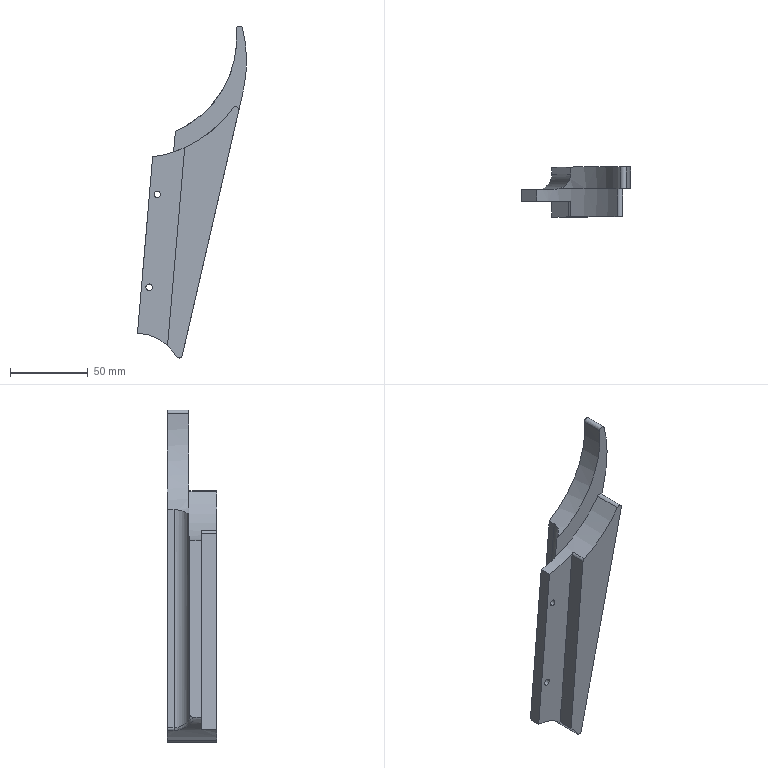Part | SolidWorks | features ICE 3, Fillet 2, DelFace 1, Extrusion 1, MirrorSolid 1 | 1 solid | 26 faces | box 70.208 x 32 x 213.495 mm | volume 127310 mm3 | cylinder 15 | plane 9 | spline 1 | torus 1 | commonest cylinder face diameters 4 x6 4.2 x4 20 x1 61 x1 130 x1 154 x1
STEP:
#1=CARTESIAN_POINT('',(13.896,-7.5,121.876));
#2=VERTEX_POINT('',#1);
#3=CARTESIAN_POINT('',(13.896,-7.5,117.676));
#4=VERTEX_POINT('',#3);
#5=CARTESIAN_POINT('',(13.896,-7.5,119.776));
#6=DIRECTION('',(0.,-1.,0.));
#7=DIRECTION('',(0.,0.,1.));
#8=AXIS2_PLACEMENT_3D('',#5,#6,#7);
#9=CIRCLE('',#8,2.1);
#10=EDGE_CURVE('',#2,#4,#9,.T.);
#11=ORIENTED_EDGE('',*,*,#10,.T.);
#12=CARTESIAN_POINT('',(13.896,0.,117.676));
#13=VERTEX_POINT('',#12);
#14=CARTESIAN_POINT('',(13.896,-148.287,117.676));
#15=DIRECTION('',(0.,1.,0.));
#16=VECTOR('',#15,1000.);
#17=LINE('',#14,#16);
#18=EDGE_CURVE('',#4,#13,#17,.T.);
#19=ORIENTED_EDGE('',*,*,#18,.T.);
#20=CARTESIAN_POINT('',(13.896,0.,121.876));
#21=VERTEX_POINT('',#20);
#22=CARTESIAN_POINT('',(13.896,0.,119.776));
#23=DIRECTION('',(0.,1.,0.));
#24=DIRECTION('',(0.,0.,1.));
#25=AXIS2_PLACEMENT_3D('',#22,#23,#24);
#26=CIRCLE('',#25,2.1);
#27=EDGE_CURVE('',#13,#21,#26,.T.);
#28=ORIENTED_EDGE('',*,*,#27,.T.);
#29=CARTESIAN_POINT('',(13.896,-148.287,121.876));
#30=DIRECTION('',(0.,1.,0.));
#31=VECTOR('',#30,1000.);
#32=LINE('',#29,#31);
#33=EDGE_CURVE('',#2,#21,#32,.T.);
#34=ORIENTED_EDGE('',*,*,#33,.F.);
#35=EDGE_LOOP('',(#11,#19,#28,#34));
#36=FACE_OUTER_BOUND('',#35,.T.);
#37=CARTESIAN_POINT('',(13.896,-148.287,119.776));
#38=DIRECTION('',(0.,1.,0.));
#39=DIRECTION('',(0.,0.,1.));
#40=AXIS2_PLACEMENT_3D('',#37,#38,#39);
#41=CYLINDRICAL_SURFACE('',#40,2.1);
#42=ADVANCED_FACE('',(#36),#41,.F.);
#43=CARTESIAN_POINT('',(8.714,-7.5,62.1));
#44=VERTEX_POINT('',#43);
#45=CARTESIAN_POINT('',(8.714,-7.5,57.9));
#46=VERTEX_POINT('',#45);
#47=CARTESIAN_POINT('',(8.714,-7.5,60.));
#48=DIRECTION('',(0.,-1.,0.));
#49=DIRECTION('',(0.,0.,1.));
#50=AXIS2_PLACEMENT_3D('',#47,#48,#49);
#51=CIRCLE('',#50,2.1);
#52=EDGE_CURVE('',#44,#46,#51,.T.);
#53=ORIENTED_EDGE('',*,*,#52,.T.);
#54=CARTESIAN_POINT('',(8.714,0.,57.9));
#55=VERTEX_POINT('',#54);
#56=CARTESIAN_POINT('',(8.714,-148.287,57.9));
#57=DIRECTION('',(0.,1.,0.));
#58=VECTOR('',#57,1000.);
#59=LINE('',#56,#58);
#60=EDGE_CURVE('',#46,#55,#59,.T.);
#61=ORIENTED_EDGE('',*,*,#60,.T.);
#62=CARTESIAN_POINT('',(8.714,0.,62.1));
#63=VERTEX_POINT('',#62);
#64=CARTESIAN_POINT('',(8.714,0.,60.));
#65=DIRECTION('',(0.,1.,0.));
#66=DIRECTION('',(0.,0.,1.));
#67=AXIS2_PLACEMENT_3D('',#64,#65,#66);
#68=CIRCLE('',#67,2.1);
#69=EDGE_CURVE('',#55,#63,#68,.T.);
#70=ORIENTED_EDGE('',*,*,#69,.T.);
#71=CARTESIAN_POINT('',(8.714,-148.287,62.1));
#72=DIRECTION('',(0.,1.,0.));
#73=VECTOR('',#72,1000.);
#74=LINE('',#71,#73);
#75=EDGE_CURVE('',#44,#63,#74,.T.);
#76=ORIENTED_EDGE('',*,*,#75,.F.);
#77=EDGE_LOOP('',(#53,#61,#70,#76));
#78=FACE_OUTER_BOUND('',#77,.T.);
#79=CARTESIAN_POINT('',(8.714,-148.287,60.));
#80=DIRECTION('',(0.,1.,0.));
#81=DIRECTION('',(0.,0.,1.));
#82=AXIS2_PLACEMENT_3D('',#79,#80,#81);
#83=CYLINDRICAL_SURFACE('',#82,2.1);
#84=ADVANCED_FACE('',(#78),#83,.F.);
#85=CARTESIAN_POINT('',(26.282,14.5,15.476));
#86=VERTEX_POINT('',#85);
#87=CARTESIAN_POINT('',(28.006,14.5,14.491));
#88=VERTEX_POINT('',#87);
#89=CARTESIAN_POINT('',(28.006,14.5,16.491));
#90=DIRECTION('',(0.,-1.,0.));
#91=DIRECTION('',(0.,0.,1.));
#92=AXIS2_PLACEMENT_3D('',#89,#90,#91);
#93=CIRCLE('',#92,2.);
#94=EDGE_CURVE('',#86,#88,#93,.T.);
#95=ORIENTED_EDGE('',*,*,#94,.T.);
#96=CARTESIAN_POINT('',(28.006,-17.5,14.491));
#97=VERTEX_POINT('',#96);
#98=CARTESIAN_POINT('',(28.006,17.5,14.491));
#99=DIRECTION('',(0.,-1.,0.));
#100=VECTOR('',#99,1000.);
#101=LINE('',#98,#100);
#102=EDGE_CURVE('',#88,#97,#101,.T.);
#103=ORIENTED_EDGE('',*,*,#102,.T.);
#104=CARTESIAN_POINT('',(26.282,-17.5,15.476));
#105=VERTEX_POINT('',#104);
#106=CARTESIAN_POINT('',(28.006,-17.5,16.491));
#107=DIRECTION('',(0.,-1.,0.));
#108=DIRECTION('',(0.,0.,1.));
#109=AXIS2_PLACEMENT_3D('',#106,#107,#108);
#110=CIRCLE('',#109,2.);
#111=EDGE_CURVE('',#105,#97,#110,.T.);
#112=ORIENTED_EDGE('',*,*,#111,.F.);
#113=CARTESIAN_POINT('',(26.282,17.5,15.476));
#114=DIRECTION('',(0.,-1.,0.));
#115=VECTOR('',#114,1000.);
#116=LINE('',#113,#115);
#117=EDGE_CURVE('',#86,#105,#116,.T.);
#118=ORIENTED_EDGE('',*,*,#117,.F.);
#119=EDGE_LOOP('',(#95,#103,#112,#118));
#120=FACE_OUTER_BOUND('',#119,.T.);
#121=CARTESIAN_POINT('',(28.006,17.5,16.491));
#122=DIRECTION('',(0.,-1.,0.));
#123=DIRECTION('',(0.,0.,-1.));
#124=AXIS2_PLACEMENT_3D('',#121,#122,#123);
#125=CYLINDRICAL_SURFACE('',#124,2.);
#126=ADVANCED_FACE('',(#120),#125,.T.);
#127=CARTESIAN_POINT('',(32.775,14.5,163.868));
#128=VERTEX_POINT('',#127);
#129=CARTESIAN_POINT('',(20.609,14.5,23.527));
#130=VERTEX_POINT('',#129);
#131=CARTESIAN_POINT('',(35.992,14.5,200.98));
#132=DIRECTION('',(-0.08636,0.,-0.9963));
#133=VECTOR('',#132,1000.);
#134=LINE('',#131,#133);
#135=EDGE_CURVE('',#128,#130,#134,.T.);
#136=ORIENTED_EDGE('',*,*,#135,.T.);
#137=CARTESIAN_POINT('',(20.609,10.,23.527));
#138=VERTEX_POINT('',#137);
#139=CARTESIAN_POINT('',(20.609,17.5,23.527));
#140=DIRECTION('',(0.,-1.,0.));
#141=VECTOR('',#140,1000.);
#142=LINE('',#139,#141);
#143=EDGE_CURVE('',#130,#138,#142,.T.);
#144=ORIENTED_EDGE('',*,*,#143,.T.);
#145=CARTESIAN_POINT('',(32.775,10.,163.868));
#146=VERTEX_POINT('',#145);
#147=CARTESIAN_POINT('',(20.525,10.,22.56));
#148=DIRECTION('',(0.08636,0.,0.9963));
#149=VECTOR('',#148,1000.);
#150=LINE('',#147,#149);
#151=EDGE_CURVE('',#138,#146,#150,.T.);
#152=ORIENTED_EDGE('',*,*,#151,.T.);
#153=CARTESIAN_POINT('',(32.775,0.5,163.868));
#154=DIRECTION('',(0.,1.,0.));
#155=VECTOR('',#154,1000.);
#156=LINE('',#153,#155);
#157=EDGE_CURVE('',#146,#128,#156,.T.);
#158=ORIENTED_EDGE('',*,*,#157,.T.);
#159=EDGE_LOOP('',(#136,#144,#152,#158));
#160=FACE_OUTER_BOUND('',#159,.T.);
#161=CARTESIAN_POINT('',(20.525,17.5,22.56));
#162=DIRECTION('',(0.9963,0.,-0.08636));
#163=DIRECTION('',(-0.08636,0.,-0.9963));
#164=AXIS2_PLACEMENT_3D('',#161,#162,#163);
#165=PLANE('',#164);
#166=ADVANCED_FACE('',(#160),#165,.F.);
#167=CARTESIAN_POINT('',(29.954,-17.5,16.041));
#168=VERTEX_POINT('',#167);
#169=CARTESIAN_POINT('',(29.954,14.5,16.041));
#170=VERTEX_POINT('',#169);
#171=CARTESIAN_POINT('',(29.954,17.5,16.041));
#172=DIRECTION('',(0.,1.,0.));
#173=VECTOR('',#172,1000.);
#174=LINE('',#171,#173);
#175=EDGE_CURVE('',#168,#170,#174,.T.);
#176=ORIENTED_EDGE('',*,*,#175,.T.);
#177=CARTESIAN_POINT('',(69.167,14.5,186.164));
#178=VERTEX_POINT('',#177);
#179=CARTESIAN_POINT('',(69.167,14.5,186.164));
#180=DIRECTION('',(0.2246,0.,0.9744));
#181=VECTOR('',#180,1000.);
#182=LINE('',#179,#181);
#183=EDGE_CURVE('',#170,#178,#182,.T.);
#184=ORIENTED_EDGE('',*,*,#183,.T.);
#185=CARTESIAN_POINT('',(69.167,0.5,186.164));
#186=VERTEX_POINT('',#185);
#187=CARTESIAN_POINT('',(69.167,0.5,186.164));
#188=DIRECTION('',(0.,1.,0.));
#189=VECTOR('',#188,1000.);
#190=LINE('',#187,#189);
#191=EDGE_CURVE('',#186,#178,#190,.T.);
#192=ORIENTED_EDGE('',*,*,#191,.F.);
#193=CARTESIAN_POINT('',(66.301,0.5,173.727));
#194=VERTEX_POINT('',#193);
#195=CARTESIAN_POINT('',(28.661,0.5,10.43));
#196=DIRECTION('',(-0.2246,0.,-0.9744));
#197=VECTOR('',#196,1000.);
#198=LINE('',#195,#197);
#199=EDGE_CURVE('',#186,#194,#198,.T.);
#200=ORIENTED_EDGE('',*,*,#199,.T.);
#201=CARTESIAN_POINT('',(66.301,-17.5,173.727));
#202=VERTEX_POINT('',#201);
#203=CARTESIAN_POINT('',(66.301,17.5,173.727));
#204=DIRECTION('',(0.,-1.,0.));
#205=VECTOR('',#204,1000.);
#206=LINE('',#203,#205);
#207=EDGE_CURVE('',#194,#202,#206,.T.);
#208=ORIENTED_EDGE('',*,*,#207,.T.);
#209=CARTESIAN_POINT('',(28.661,-17.5,10.43));
#210=DIRECTION('',(-0.2246,0.,-0.9744));
#211=VECTOR('',#210,1000.);
#212=LINE('',#209,#211);
#213=EDGE_CURVE('',#202,#168,#212,.T.);
#214=ORIENTED_EDGE('',*,*,#213,.T.);
#215=EDGE_LOOP('',(#176,#184,#192,#200,#208,#214));
#216=FACE_OUTER_BOUND('',#215,.T.);
#217=CARTESIAN_POINT('',(28.661,17.5,10.43));
#218=DIRECTION('',(-0.9744,0.,0.2246));
#219=DIRECTION('',(0.2246,0.,0.9744));
#220=AXIS2_PLACEMENT_3D('',#217,#218,#219);
#221=PLANE('',#220);
#222=ADVANCED_FACE('',(#216),#221,.F.);
#223=CARTESIAN_POINT('',(21.211,14.5,21.917));
#224=VERTEX_POINT('',#223);
#225=CARTESIAN_POINT('',(0.,14.5,0.));
#226=DIRECTION('',(0.,1.,0.));
#227=DIRECTION('',(0.,0.,1.));
#228=AXIS2_PLACEMENT_3D('',#225,#226,#227);
#229=CIRCLE('',#228,30.5);
#230=EDGE_CURVE('',#224,#86,#229,.T.);
#231=ORIENTED_EDGE('',*,*,#230,.T.);
#232=ORIENTED_EDGE('',*,*,#117,.T.);
#233=CARTESIAN_POINT('',(20.525,-17.5,22.56));
#234=VERTEX_POINT('',#233);
#235=CARTESIAN_POINT('',(0.,-17.5,0.));
#236=DIRECTION('',(0.,-1.,0.));
#237=DIRECTION('',(0.,0.,1.));
#238=AXIS2_PLACEMENT_3D('',#235,#236,#237);
#239=CIRCLE('',#238,30.5);
#240=EDGE_CURVE('',#105,#234,#239,.T.);
#241=ORIENTED_EDGE('',*,*,#240,.T.);
#242=CARTESIAN_POINT('',(20.525,-7.5,22.56));
#243=VERTEX_POINT('',#242);
#244=CARTESIAN_POINT('',(20.525,17.5,22.56));
#245=DIRECTION('',(0.,-1.,0.));
#246=VECTOR('',#245,1000.);
#247=LINE('',#244,#246);
#248=EDGE_CURVE('',#243,#234,#247,.T.);
#249=ORIENTED_EDGE('',*,*,#248,.F.);
#250=CARTESIAN_POINT('',(1.137,-7.5,30.479));
#251=VERTEX_POINT('',#250);
#252=CARTESIAN_POINT('',(0.,-7.5,0.));
#253=DIRECTION('',(0.,1.,0.));
#254=DIRECTION('',(0.,0.,1.));
#255=AXIS2_PLACEMENT_3D('',#252,#253,#254);
#256=CIRCLE('',#255,30.5);
#257=EDGE_CURVE('',#251,#243,#256,.T.);
#258=ORIENTED_EDGE('',*,*,#257,.F.);
#259=CARTESIAN_POINT('',(1.137,-2.,30.479));
#260=VERTEX_POINT('',#259);
#261=CARTESIAN_POINT('',(1.137,-148.287,30.479));
#262=DIRECTION('',(0.,1.,0.));
#263=VECTOR('',#262,1000.);
#264=LINE('',#261,#263);
#265=EDGE_CURVE('',#251,#260,#264,.T.);
#266=ORIENTED_EDGE('',*,*,#265,.T.);
#267=CARTESIAN_POINT('',(10.49,-2.,28.639));
#268=VERTEX_POINT('',#267);
#269=CARTESIAN_POINT('',(0.,-2.,0.));
#270=DIRECTION('',(0.,1.,0.));
#271=DIRECTION('',(0.,0.,1.));
#272=AXIS2_PLACEMENT_3D('',#269,#270,#271);
#273=CIRCLE('',#272,30.5);
#274=EDGE_CURVE('',#260,#268,#273,.T.);
#275=ORIENTED_EDGE('',*,*,#274,.T.);
#276=CARTESIAN_POINT('',(21.211,10.,21.917));
#277=VERTEX_POINT('',#276);
#278=CARTESIAN_POINT('',(10.49,-2.,28.639));
#279=CARTESIAN_POINT('',(11.252,-2.,28.36));
#280=CARTESIAN_POINT('',(11.986,-1.914,28.057));
#281=CARTESIAN_POINT('',(13.052,-1.671,27.569));
#282=CARTESIAN_POINT('',(13.401,-1.571,27.401));
#283=CARTESIAN_POINT('',(14.087,-1.333,27.054));
#284=CARTESIAN_POINT('',(14.425,-1.194,26.876));
#285=CARTESIAN_POINT('',(15.401,-0.7323,26.337));
#286=CARTESIAN_POINT('',(16.007,-0.3609,25.971));
#287=CARTESIAN_POINT('',(16.858,0.2868,25.42));
#288=CARTESIAN_POINT('',(17.133,0.5188,25.235));
#289=CARTESIAN_POINT('',(17.659,1.01,24.87));
#290=CARTESIAN_POINT('',(17.909,1.268,24.69));
#291=CARTESIAN_POINT('',(18.621,2.077,24.163));
#292=CARTESIAN_POINT('',(19.046,2.663,23.827));
#293=CARTESIAN_POINT('',(19.611,3.618,23.36));
#294=CARTESIAN_POINT('',(19.789,3.951,23.21));
#295=CARTESIAN_POINT('',(20.112,4.635,22.93));
#296=CARTESIAN_POINT('',(20.259,4.985,22.8));
#297=CARTESIAN_POINT('',(20.523,5.703,22.563));
#298=CARTESIAN_POINT('',(20.641,6.071,22.455));
#299=CARTESIAN_POINT('',(20.844,6.825,22.266));
#300=CARTESIAN_POINT('',(20.931,7.214,22.184));
#301=CARTESIAN_POINT('',(21.14,8.391,21.986));
#302=CARTESIAN_POINT('',(21.211,9.188,21.917));
#303=CARTESIAN_POINT('',(21.211,10.,21.917));
#304=B_SPLINE_CURVE_WITH_KNOTS('',3,(#278,#279,#280,#281,#282,#283,#284,#285,#286,#287,#288,#289,#290,#291,#292,#293,#294,#295,#296,#297,#298,#299,#300,#301,#302,#303),.UNSPECIFIED.,.F.,.F.,(4,2,2,2,2,2,2,2,2,2,2,2,4),(0.,0.002393,0.003589,0.004785,0.007178,0.008374,0.009571,0.01196,0.01316,0.01436,0.01555,0.01675,0.01914),.UNSPECIFIED.);
#305=EDGE_CURVE('',#268,#277,#304,.T.);
#306=ORIENTED_EDGE('',*,*,#305,.T.);
#307=CARTESIAN_POINT('',(21.211,17.5,21.917));
#308=DIRECTION('',(0.,1.,0.));
#309=VECTOR('',#308,1000.);
#310=LINE('',#307,#309);
#311=EDGE_CURVE('',#277,#224,#310,.T.);
#312=ORIENTED_EDGE('',*,*,#311,.T.);
#313=EDGE_LOOP('',(#231,#232,#241,#249,#258,#266,#275,#306,#312));
#314=FACE_OUTER_BOUND('',#313,.T.);
#315=CARTESIAN_POINT('',(0.,17.5,0.));
#316=DIRECTION('',(0.,-1.,0.));
#317=DIRECTION('',(0.,0.,-1.));
#318=AXIS2_PLACEMENT_3D('',#315,#316,#317);
#319=CYLINDRICAL_SURFACE('',#318,30.5);
#320=ADVANCED_FACE('',(#314),#319,.F.);
#321=ORIENTED_EDGE('',*,*,#143,.F.);
#322=CARTESIAN_POINT('',(22.601,14.5,23.354));
#323=DIRECTION('',(0.,-1.,0.));
#324=DIRECTION('',(0.,0.,1.));
#325=AXIS2_PLACEMENT_3D('',#322,#323,#324);
#326=CIRCLE('',#325,2.);
#327=EDGE_CURVE('',#130,#224,#326,.T.);
#328=ORIENTED_EDGE('',*,*,#327,.T.);
#329=ORIENTED_EDGE('',*,*,#311,.F.);
#330=CARTESIAN_POINT('',(22.601,10.,23.354));
#331=DIRECTION('',(0.,-1.,0.));
#332=DIRECTION('',(0.,0.,-1.));
#333=AXIS2_PLACEMENT_3D('',#330,#331,#332);
#334=CIRCLE('',#333,2.);
#335=EDGE_CURVE('',#138,#277,#334,.T.);
#336=ORIENTED_EDGE('',*,*,#335,.F.);
#337=EDGE_LOOP('',(#321,#328,#329,#336));
#338=FACE_OUTER_BOUND('',#337,.T.);
#339=CARTESIAN_POINT('',(22.601,17.5,23.354));
#340=DIRECTION('',(0.,-1.,0.));
#341=DIRECTION('',(0.,0.,-1.));
#342=AXIS2_PLACEMENT_3D('',#339,#340,#341);
#343=CYLINDRICAL_SURFACE('',#342,2.);
#344=ADVANCED_FACE('',(#338),#343,.T.);
#345=ORIENTED_EDGE('',*,*,#102,.F.);
#346=CARTESIAN_POINT('',(28.006,14.5,16.491));
#347=DIRECTION('',(0.,-1.,0.));
#348=DIRECTION('',(0.,0.,1.));
#349=AXIS2_PLACEMENT_3D('',#346,#347,#348);
#350=CIRCLE('',#349,2.);
#351=EDGE_CURVE('',#88,#170,#350,.T.);
#352=ORIENTED_EDGE('',*,*,#351,.T.);
#353=ORIENTED_EDGE('',*,*,#175,.F.);
#354=CARTESIAN_POINT('',(28.006,-17.5,16.491));
#355=DIRECTION('',(0.,-1.,0.));
#356=DIRECTION('',(0.,0.,1.));
#357=AXIS2_PLACEMENT_3D('',#354,#355,#356);
#358=CIRCLE('',#357,2.);
#359=EDGE_CURVE('',#97,#168,#358,.T.);
#360=ORIENTED_EDGE('',*,*,#359,.F.);
#361=EDGE_LOOP('',(#345,#352,#353,#360));
#362=FACE_OUTER_BOUND('',#361,.T.);
#363=CARTESIAN_POINT('',(28.006,17.5,16.491));
#364=DIRECTION('',(0.,-1.,0.));
#365=DIRECTION('',(0.,0.,-1.));
#366=AXIS2_PLACEMENT_3D('',#363,#364,#365);
#367=CYLINDRICAL_SURFACE('',#366,2.);
#368=ADVANCED_FACE('',(#362),#367,.T.);
#369=CARTESIAN_POINT('',(32.597,-17.5,150.24));
#370=VERTEX_POINT('',#369);
#371=CARTESIAN_POINT('',(62.723,-17.5,175.336));
#372=VERTEX_POINT('',#371);
#373=CARTESIAN_POINT('',(0.,-17.5,220.));
#374=DIRECTION('',(0.,-1.,0.));
#375=DIRECTION('',(0.,0.,1.));
#376=AXIS2_PLACEMENT_3D('',#373,#374,#375);
#377=CIRCLE('',#376,77.);
#378=EDGE_CURVE('',#370,#372,#377,.T.);
#379=ORIENTED_EDGE('',*,*,#378,.T.);
#380=CARTESIAN_POINT('',(62.723,0.5,175.336));
#381=VERTEX_POINT('',#380);
#382=CARTESIAN_POINT('',(62.723,17.5,175.336));
#383=DIRECTION('',(0.,1.,0.));
#384=VECTOR('',#383,1000.);
#385=LINE('',#382,#384);
#386=EDGE_CURVE('',#372,#381,#385,.T.);
#387=ORIENTED_EDGE('',*,*,#386,.T.);
#388=CARTESIAN_POINT('',(24.407,0.5,146.97));
#389=VERTEX_POINT('',#388);
#390=CARTESIAN_POINT('',(0.,0.5,220.));
#391=DIRECTION('',(0.,1.,0.));
#392=DIRECTION('',(0.,0.,1.));
#393=AXIS2_PLACEMENT_3D('',#390,#391,#392);
#394=CIRCLE('',#393,77.);
#395=EDGE_CURVE('',#381,#389,#394,.T.);
#396=ORIENTED_EDGE('',*,*,#395,.T.);
#397=CARTESIAN_POINT('',(21.186,0.,145.972));
#398=VERTEX_POINT('',#397);
#399=CARTESIAN_POINT('',(24.407,0.5,146.97));
#400=CARTESIAN_POINT('',(23.364,0.1684,146.622));
#401=CARTESIAN_POINT('',(22.291,0.,146.288));
#402=CARTESIAN_POINT('',(21.186,0.,145.972));
#403=B_SPLINE_CURVE_WITH_KNOTS('',3,(#399,#400,#401,#402),.UNSPECIFIED.,.F.,.F.,(4,4),(0.01301,0.01641),.UNSPECIFIED.);
#404=EDGE_CURVE('',#389,#398,#403,.T.);
#405=ORIENTED_EDGE('',*,*,#404,.T.);
#406=CARTESIAN_POINT('',(10.959,0.,143.784));
#407=VERTEX_POINT('',#406);
#408=CARTESIAN_POINT('',(0.,0.,220.));
#409=DIRECTION('',(0.,-1.,0.));
#410=DIRECTION('',(0.,0.,1.));
#411=AXIS2_PLACEMENT_3D('',#408,#409,#410);
#412=CIRCLE('',#411,77.);
#413=EDGE_CURVE('',#407,#398,#412,.T.);
#414=ORIENTED_EDGE('',*,*,#413,.F.);
#415=CARTESIAN_POINT('',(10.959,-7.5,143.784));
#416=VERTEX_POINT('',#415);
#417=CARTESIAN_POINT('',(10.959,-148.287,143.784));
#418=DIRECTION('',(0.,1.,0.));
#419=VECTOR('',#418,1000.);
#420=LINE('',#417,#419);
#421=EDGE_CURVE('',#416,#407,#420,.T.);
#422=ORIENTED_EDGE('',*,*,#421,.F.);
#423=CARTESIAN_POINT('',(32.597,-7.5,150.24));
#424=VERTEX_POINT('',#423);
#425=CARTESIAN_POINT('',(0.,-7.5,220.));
#426=DIRECTION('',(0.,1.,0.));
#427=DIRECTION('',(0.,0.,1.));
#428=AXIS2_PLACEMENT_3D('',#425,#426,#427);
#429=CIRCLE('',#428,77.);
#430=EDGE_CURVE('',#424,#416,#429,.T.);
#431=ORIENTED_EDGE('',*,*,#430,.F.);
#432=CARTESIAN_POINT('',(32.597,17.5,150.24));
#433=DIRECTION('',(0.,-1.,0.));
#434=VECTOR('',#433,1000.);
#435=LINE('',#432,#434);
#436=EDGE_CURVE('',#424,#370,#435,.T.);
#437=ORIENTED_EDGE('',*,*,#436,.T.);
#438=EDGE_LOOP('',(#379,#387,#396,#405,#414,#422,#431,#437));
#439=FACE_OUTER_BOUND('',#438,.T.);
#440=CARTESIAN_POINT('',(0.,17.5,220.));
#441=DIRECTION('',(0.,-1.,0.));
#442=DIRECTION('',(0.,0.,-1.));
#443=AXIS2_PLACEMENT_3D('',#440,#441,#442);
#444=CYLINDRICAL_SURFACE('',#443,77.);
#445=ADVANCED_FACE('',(#439),#444,.F.);
#446=CARTESIAN_POINT('',(31.451,-17.5,148.601));
#447=VERTEX_POINT('',#446);
#448=CARTESIAN_POINT('',(20.525,-17.5,22.56));
#449=DIRECTION('',(0.08636,0.,0.9963));
#450=VECTOR('',#449,1000.);
#451=LINE('',#448,#450);
#452=EDGE_CURVE('',#234,#447,#451,.T.);
#453=ORIENTED_EDGE('',*,*,#452,.T.);
#454=CARTESIAN_POINT('',(31.451,-7.5,148.601));
#455=VERTEX_POINT('',#454);
#456=CARTESIAN_POINT('',(31.451,17.5,148.601));
#457=DIRECTION('',(0.,1.,0.));
#458=VECTOR('',#457,1000.);
#459=LINE('',#456,#458);
#460=EDGE_CURVE('',#447,#455,#459,.T.);
#461=ORIENTED_EDGE('',*,*,#460,.T.);
#462=CARTESIAN_POINT('',(20.525,-7.5,22.56));
#463=DIRECTION('',(0.08636,0.,0.9963));
#464=VECTOR('',#463,1000.);
#465=LINE('',#462,#464);
#466=EDGE_CURVE('',#243,#455,#465,.T.);
#467=ORIENTED_EDGE('',*,*,#466,.F.);
#468=ORIENTED_EDGE('',*,*,#248,.T.);
#469=EDGE_LOOP('',(#453,#461,#467,#468));
#470=FACE_OUTER_BOUND('',#469,.T.);
#471=CARTESIAN_POINT('',(20.525,17.5,22.56));
#472=DIRECTION('',(0.9963,0.,-0.08636));
#473=DIRECTION('',(-0.08636,0.,-0.9963));
#474=AXIS2_PLACEMENT_3D('',#471,#472,#473);
#475=PLANE('',#474);
#476=ADVANCED_FACE('',(#470),#475,.F.);
#477=ORIENTED_EDGE('',*,*,#213,.F.);
#478=CARTESIAN_POINT('',(64.352,-17.5,174.176));
#479=DIRECTION('',(0.,-1.,0.));
#480=DIRECTION('',(0.,0.,1.));
#481=AXIS2_PLACEMENT_3D('',#478,#479,#480);
#482=CIRCLE('',#481,2.);
#483=EDGE_CURVE('',#202,#372,#482,.T.);
#484=ORIENTED_EDGE('',*,*,#483,.T.);
#485=ORIENTED_EDGE('',*,*,#378,.F.);
#486=CARTESIAN_POINT('',(33.444,-17.5,148.428));
#487=DIRECTION('',(0.,-1.,0.));
#488=DIRECTION('',(0.,0.,1.));
#489=AXIS2_PLACEMENT_3D('',#486,#487,#488);
#490=CIRCLE('',#489,2.);
#491=EDGE_CURVE('',#370,#447,#490,.T.);
#492=ORIENTED_EDGE('',*,*,#491,.T.);
#493=ORIENTED_EDGE('',*,*,#452,.F.);
#494=ORIENTED_EDGE('',*,*,#240,.F.);
#495=ORIENTED_EDGE('',*,*,#111,.T.);
#496=ORIENTED_EDGE('',*,*,#359,.T.);
#497=EDGE_LOOP('',(#477,#484,#485,#492,#493,#494,#495,#496));
#498=FACE_OUTER_BOUND('',#497,.T.);
#499=CARTESIAN_POINT('',(0.,-17.5,220.));
#500=DIRECTION('',(0.,1.,0.));
#501=DIRECTION('',(0.,0.,1.));
#502=AXIS2_PLACEMENT_3D('',#499,#500,#501);
#503=PLANE('',#502);
#504=ADVANCED_FACE('',(#498),#503,.F.);
#505=CARTESIAN_POINT('',(1.309,0.,32.474));
#506=VERTEX_POINT('',#505);
#507=CARTESIAN_POINT('',(1.137,0.,30.479));
#508=DIRECTION('',(0.08636,0.,0.9963));
#509=VECTOR('',#508,1000.);
#510=LINE('',#507,#509);
#511=EDGE_CURVE('',#506,#407,#510,.T.);
#512=ORIENTED_EDGE('',*,*,#511,.F.);
#513=CARTESIAN_POINT('',(1.309,0.,32.474));
#514=CARTESIAN_POINT('',(1.298,0.,32.342));
#515=CARTESIAN_POINT('',(1.287,-0.01294,32.213));
#516=CARTESIAN_POINT('',(1.265,-0.06363,31.958));
#517=CARTESIAN_POINT('',(1.254,-0.102,31.831));
#518=CARTESIAN_POINT('',(1.233,-0.2022,31.59));
#519=CARTESIAN_POINT('',(1.223,-0.2635,31.475));
#520=CARTESIAN_POINT('',(1.204,-0.4084,31.259));
#521=CARTESIAN_POINT('',(1.195,-0.4927,31.156));
#522=CARTESIAN_POINT('',(1.171,-0.7692,30.88));
#523=CARTESIAN_POINT('',(1.158,-0.9921,30.731));
#524=CARTESIAN_POINT('',(1.141,-1.473,30.532));
#525=CARTESIAN_POINT('',(1.137,-1.736,30.479));
#526=CARTESIAN_POINT('',(1.137,-2.,30.479));
#527=B_SPLINE_CURVE_WITH_KNOTS('',3,(#513,#514,#515,#516,#517,#518,#519,#520,#521,#522,#523,#524,#525,#526),.UNSPECIFIED.,.F.,.F.,(4,2,2,2,2,2,4),(0.,0.0003908,0.0007815,0.001172,0.001563,0.002345,0.003126),.UNSPECIFIED.);
#528=EDGE_CURVE('',#506,#260,#527,.T.);
#529=ORIENTED_EDGE('',*,*,#528,.T.);
#530=ORIENTED_EDGE('',*,*,#265,.F.);
#531=CARTESIAN_POINT('',(1.137,-7.5,30.479));
#532=DIRECTION('',(-0.08636,0.,-0.9963));
#533=VECTOR('',#532,1000.);
#534=LINE('',#531,#533);
#535=EDGE_CURVE('',#416,#251,#534,.T.);
#536=ORIENTED_EDGE('',*,*,#535,.F.);
#537=ORIENTED_EDGE('',*,*,#421,.T.);
#538=EDGE_LOOP('',(#512,#529,#530,#536,#537));
#539=FACE_OUTER_BOUND('',#538,.T.);
#540=CARTESIAN_POINT('',(1.137,-148.287,30.479));
#541=DIRECTION('',(-0.9963,0.,0.08636));
#542=DIRECTION('',(0.08636,0.,0.9963));
#543=AXIS2_PLACEMENT_3D('',#540,#541,#542);
#544=PLANE('',#543);
#545=ADVANCED_FACE('',(#539),#544,.T.);
#546=ORIENTED_EDGE('',*,*,#60,.F.);
#547=CARTESIAN_POINT('',(8.714,-7.5,60.));
#548=DIRECTION('',(0.,-1.,0.));
#549=DIRECTION('',(0.,0.,1.));
#550=AXIS2_PLACEMENT_3D('',#547,#548,#549);
#551=CIRCLE('',#550,2.1);
#552=EDGE_CURVE('',#46,#44,#551,.T.);
#553=ORIENTED_EDGE('',*,*,#552,.T.);
#554=ORIENTED_EDGE('',*,*,#75,.T.);
#555=CARTESIAN_POINT('',(8.714,0.,60.));
#556=DIRECTION('',(0.,1.,0.));
#557=DIRECTION('',(0.,0.,1.));
#558=AXIS2_PLACEMENT_3D('',#555,#556,#557);
#559=CIRCLE('',#558,2.1);
#560=EDGE_CURVE('',#63,#55,#559,.T.);
#561=ORIENTED_EDGE('',*,*,#560,.T.);
#562=EDGE_LOOP('',(#546,#553,#554,#561));
#563=FACE_OUTER_BOUND('',#562,.T.);
#564=CARTESIAN_POINT('',(8.714,-148.287,60.));
#565=DIRECTION('',(0.,1.,0.));
#566=DIRECTION('',(0.,0.,1.));
#567=AXIS2_PLACEMENT_3D('',#564,#565,#566);
#568=CYLINDRICAL_SURFACE('',#567,2.1);
#569=ADVANCED_FACE('',(#563),#568,.F.);
#570=CARTESIAN_POINT('',(13.896,0.,119.776));
#571=DIRECTION('',(0.,1.,0.));
#572=DIRECTION('',(0.,0.,1.));
#573=AXIS2_PLACEMENT_3D('',#570,#571,#572);
#574=CIRCLE('',#573,2.1);
#575=EDGE_CURVE('',#21,#13,#574,.T.);
#576=ORIENTED_EDGE('',*,*,#575,.F.);
#577=ORIENTED_EDGE('',*,*,#27,.F.);
#578=EDGE_LOOP('',(#576,#577));
#579=FACE_BOUND('',#578,.T.);
#580=ORIENTED_EDGE('',*,*,#560,.F.);
#581=ORIENTED_EDGE('',*,*,#69,.F.);
#582=EDGE_LOOP('',(#580,#581));
#583=FACE_BOUND('',#582,.T.);
#584=CARTESIAN_POINT('',(11.177,0.,30.517));
#585=VERTEX_POINT('',#584);
#586=CARTESIAN_POINT('',(8.468,0.,-0.7341));
#587=DIRECTION('',(-0.08636,0.,-0.9963));
#588=VECTOR('',#587,1000.);
#589=LINE('',#586,#588);
#590=EDGE_CURVE('',#398,#585,#589,.T.);
#591=ORIENTED_EDGE('',*,*,#590,.T.);
#592=CARTESIAN_POINT('',(0.,0.,0.));
#593=DIRECTION('',(0.,-1.,0.));
#594=DIRECTION('',(0.,0.,1.));
#595=AXIS2_PLACEMENT_3D('',#592,#593,#594);
#596=CIRCLE('',#595,32.5);
#597=EDGE_CURVE('',#585,#506,#596,.T.);
#598=ORIENTED_EDGE('',*,*,#597,.T.);
#599=ORIENTED_EDGE('',*,*,#511,.T.);
#600=ORIENTED_EDGE('',*,*,#413,.T.);
#601=EDGE_LOOP('',(#591,#598,#599,#600));
#602=FACE_OUTER_BOUND('',#601,.T.);
#603=CARTESIAN_POINT('',(0.,0.,0.));
#604=DIRECTION('',(0.,1.,0.));
#605=DIRECTION('',(0.,0.,1.));
#606=AXIS2_PLACEMENT_3D('',#603,#604,#605);
#607=PLANE('',#606);
#608=ADVANCED_FACE('',(#579,#583,#602),#607,.T.);
#609=ORIENTED_EDGE('',*,*,#18,.F.);
#610=CARTESIAN_POINT('',(13.896,-7.5,119.776));
#611=DIRECTION('',(0.,-1.,0.));
#612=DIRECTION('',(0.,0.,1.));
#613=AXIS2_PLACEMENT_3D('',#610,#611,#612);
#614=CIRCLE('',#613,2.1);
#615=EDGE_CURVE('',#4,#2,#614,.T.);
#616=ORIENTED_EDGE('',*,*,#615,.T.);
#617=ORIENTED_EDGE('',*,*,#33,.T.);
#618=ORIENTED_EDGE('',*,*,#575,.T.);
#619=EDGE_LOOP('',(#609,#616,#617,#618));
#620=FACE_OUTER_BOUND('',#619,.T.);
#621=CARTESIAN_POINT('',(13.896,-148.287,119.776));
#622=DIRECTION('',(0.,1.,0.));
#623=DIRECTION('',(0.,0.,1.));
#624=AXIS2_PLACEMENT_3D('',#621,#622,#623);
#625=CYLINDRICAL_SURFACE('',#624,2.1);
#626=ADVANCED_FACE('',(#620),#625,.F.);
#627=ORIENTED_EDGE('',*,*,#257,.T.);
#628=ORIENTED_EDGE('',*,*,#466,.T.);
#629=CARTESIAN_POINT('',(33.444,-7.5,148.428));
#630=DIRECTION('',(0.,1.,0.));
#631=DIRECTION('',(0.,0.,1.));
#632=AXIS2_PLACEMENT_3D('',#629,#630,#631);
#633=CIRCLE('',#632,2.);
#634=EDGE_CURVE('',#455,#424,#633,.T.);
#635=ORIENTED_EDGE('',*,*,#634,.T.);
#636=ORIENTED_EDGE('',*,*,#430,.T.);
#637=ORIENTED_EDGE('',*,*,#535,.T.);
#638=EDGE_LOOP('',(#627,#628,#635,#636,#637));
#639=FACE_OUTER_BOUND('',#638,.T.);
#640=ORIENTED_EDGE('',*,*,#10,.F.);
#641=ORIENTED_EDGE('',*,*,#615,.F.);
#642=EDGE_LOOP('',(#640,#641));
#643=FACE_BOUND('',#642,.T.);
#644=ORIENTED_EDGE('',*,*,#52,.F.);
#645=ORIENTED_EDGE('',*,*,#552,.F.);
#646=EDGE_LOOP('',(#644,#645));
#647=FACE_BOUND('',#646,.T.);
#648=CARTESIAN_POINT('',(0.,-7.5,220.));
#649=DIRECTION('',(0.,1.,0.));
#650=DIRECTION('',(0.,0.,1.));
#651=AXIS2_PLACEMENT_3D('',#648,#649,#650);
#652=PLANE('',#651);
#653=ADVANCED_FACE('',(#639,#643,#647),#652,.F.);
#654=ORIENTED_EDGE('',*,*,#151,.F.);
#655=CARTESIAN_POINT('',(20.609,10.,23.527));
#656=CARTESIAN_POINT('',(20.609,9.283,23.527));
#657=CARTESIAN_POINT('',(20.539,8.582,23.609));
#658=CARTESIAN_POINT('',(20.338,7.556,23.837));
#659=CARTESIAN_POINT('',(20.254,7.22,23.931));
#660=CARTESIAN_POINT('',(20.061,6.574,24.145));
#661=CARTESIAN_POINT('',(19.951,6.261,24.265));
#662=CARTESIAN_POINT('',(19.704,5.654,24.528));
#663=CARTESIAN_POINT('',(19.568,5.36,24.671));
#664=CARTESIAN_POINT('',(19.27,4.788,24.977));
#665=CARTESIAN_POINT('',(19.109,4.514,25.138));
#666=CARTESIAN_POINT('',(18.599,3.729,25.635));
#667=CARTESIAN_POINT('',(18.219,3.252,25.988));
#668=CARTESIAN_POINT('',(17.38,2.381,26.718));
#669=CARTESIAN_POINT('',(16.916,1.985,27.097));
#670=CARTESIAN_POINT('',(15.931,1.298,27.843));
#671=CARTESIAN_POINT('',(15.407,1.004,28.212));
#672=CARTESIAN_POINT('',(14.566,0.6377,28.753));
#673=CARTESIAN_POINT('',(14.275,0.5283,28.932));
#674=CARTESIAN_POINT('',(13.686,0.3402,29.279));
#675=CARTESIAN_POINT('',(13.386,0.261,29.447));
#676=CARTESIAN_POINT('',(12.469,0.06853,29.935));
#677=CARTESIAN_POINT('',(11.836,0.,30.238));
#678=CARTESIAN_POINT('',(11.177,0.,30.517));
#679=B_SPLINE_CURVE_WITH_KNOTS('',3,(#655,#656,#657,#658,#659,#660,#661,#662,#663,#664,#665,#666,#667,#668,#669,#670,#671,#672,#673,#674,#675,#676,#677,#678),.UNSPECIFIED.,.F.,.F.,(4,2,2,2,2,2,2,2,2,2,2,4),(0.,0.002125,0.003187,0.004249,0.005311,0.006374,0.008498,0.01062,0.01275,0.01381,0.01487,0.017),.UNSPECIFIED.);
#680=EDGE_CURVE('',#138,#585,#679,.T.);
#681=ORIENTED_EDGE('',*,*,#680,.T.);
#682=ORIENTED_EDGE('',*,*,#590,.F.);
#683=ORIENTED_EDGE('',*,*,#404,.F.);
#684=CARTESIAN_POINT('',(25.556,0.5,160.235));
#685=VERTEX_POINT('',#684);
#686=CARTESIAN_POINT('',(11.579,0.5,-1.004));
#687=DIRECTION('',(0.08636,0.,0.9963));
#688=VECTOR('',#687,1000.);
#689=LINE('',#686,#688);
#690=EDGE_CURVE('',#389,#685,#689,.T.);
#691=ORIENTED_EDGE('',*,*,#690,.T.);
#692=CARTESIAN_POINT('',(25.556,0.5,160.235));
#693=CARTESIAN_POINT('',(26.546,0.8121,160.658));
#694=CARTESIAN_POINT('',(27.469,1.256,161.082));
#695=CARTESIAN_POINT('',(28.542,1.981,161.602));
#696=CARTESIAN_POINT('',(28.753,2.135,161.705));
#697=CARTESIAN_POINT('',(29.161,2.456,161.908));
#698=CARTESIAN_POINT('',(29.359,2.625,162.008));
#699=CARTESIAN_POINT('',(29.933,3.152,162.301));
#700=CARTESIAN_POINT('',(30.291,3.533,162.488));
#701=CARTESIAN_POINT('',(30.788,4.154,162.754));
#702=CARTESIAN_POINT('',(30.947,4.369,162.84));
#703=CARTESIAN_POINT('',(31.246,4.811,163.003));
#704=CARTESIAN_POINT('',(31.387,5.037,163.08));
#705=CARTESIAN_POINT('',(31.651,5.504,163.227));
#706=CARTESIAN_POINT('',(31.774,5.743,163.295));
#707=CARTESIAN_POINT('',(32.001,6.235,163.423));
#708=CARTESIAN_POINT('',(32.106,6.489,163.483));
#709=CARTESIAN_POINT('',(32.388,7.264,163.643));
#710=CARTESIAN_POINT('',(32.531,7.794,163.726));
#711=CARTESIAN_POINT('',(32.676,8.609,163.81));
#712=CARTESIAN_POINT('',(32.713,8.885,163.832));
#713=CARTESIAN_POINT('',(32.762,9.442,163.861));
#714=CARTESIAN_POINT('',(32.775,9.723,163.868));
#715=CARTESIAN_POINT('',(32.775,10.,163.868));
#716=B_SPLINE_CURVE_WITH_KNOTS('',3,(#692,#693,#694,#695,#696,#697,#698,#699,#700,#701,#702,#703,#704,#705,#706,#707,#708,#709,#710,#711,#712,#713,#714,#715),.UNSPECIFIED.,.F.,.F.,(4,2,2,2,2,2,2,2,2,2,2,4),(0.007444,0.01078,0.01161,0.01244,0.01411,0.01494,0.01577,0.01661,0.01744,0.01911,0.01994,0.02077),.UNSPECIFIED.);
#717=EDGE_CURVE('',#685,#146,#716,.T.);
#718=ORIENTED_EDGE('',*,*,#717,.T.);
#719=EDGE_LOOP('',(#654,#681,#682,#683,#691,#718));
#720=FACE_OUTER_BOUND('',#719,.T.);
#721=CARTESIAN_POINT('',(8.468,10.,-0.7341));
#722=DIRECTION('',(-0.08636,0.,-0.9963));
#723=DIRECTION('',(-0.9963,0.,0.08636));
#724=AXIS2_PLACEMENT_3D('',#721,#722,#723);
#725=CYLINDRICAL_SURFACE('',#724,10.);
#726=ADVANCED_FACE('',(#720),#725,.F.);
#727=CARTESIAN_POINT('',(68.669,14.5,226.483));
#728=VERTEX_POINT('',#727);
#729=CARTESIAN_POINT('',(-13.856,14.5,205.301));
#730=DIRECTION('',(0.,1.,0.));
#731=DIRECTION('',(0.,0.,1.));
#732=AXIS2_PLACEMENT_3D('',#729,#730,#731);
#733=CIRCLE('',#732,85.2);
#734=EDGE_CURVE('',#728,#178,#733,.T.);
#735=ORIENTED_EDGE('',*,*,#734,.F.);
#736=CARTESIAN_POINT('',(68.669,0.5,226.483));
#737=VERTEX_POINT('',#736);
#738=CARTESIAN_POINT('',(68.669,0.5,226.483));
#739=DIRECTION('',(0.,-1.,0.));
#740=VECTOR('',#739,1000.);
#741=LINE('',#738,#740);
#742=EDGE_CURVE('',#728,#737,#741,.T.);
#743=ORIENTED_EDGE('',*,*,#742,.T.);
#744=CARTESIAN_POINT('',(-13.856,0.5,205.301));
#745=DIRECTION('',(0.,1.,0.));
#746=DIRECTION('',(0.,0.,1.));
#747=AXIS2_PLACEMENT_3D('',#744,#745,#746);
#748=CIRCLE('',#747,85.2);
#749=EDGE_CURVE('',#737,#186,#748,.T.);
#750=ORIENTED_EDGE('',*,*,#749,.T.);
#751=ORIENTED_EDGE('',*,*,#191,.T.);
#752=EDGE_LOOP('',(#735,#743,#750,#751));
#753=FACE_OUTER_BOUND('',#752,.T.);
#754=CARTESIAN_POINT('',(-13.856,0.5,205.301));
#755=DIRECTION('',(0.,1.,0.));
#756=DIRECTION('',(0.,0.,1.));
#757=AXIS2_PLACEMENT_3D('',#754,#755,#756);
#758=CYLINDRICAL_SURFACE('',#757,85.2);
#759=ADVANCED_FACE('',(#753),#758,.T.);
#760=CARTESIAN_POINT('',(64.74,14.5,225.807));
#761=VERTEX_POINT('',#760);
#762=CARTESIAN_POINT('',(0.,14.5,220.));
#763=DIRECTION('',(0.,-1.,0.));
#764=DIRECTION('',(0.,0.,1.));
#765=AXIS2_PLACEMENT_3D('',#762,#763,#764);
#766=CIRCLE('',#765,65.);
#767=EDGE_CURVE('',#128,#761,#766,.T.);
#768=ORIENTED_EDGE('',*,*,#767,.F.);
#769=ORIENTED_EDGE('',*,*,#157,.F.);
#770=ORIENTED_EDGE('',*,*,#717,.F.);
#771=CARTESIAN_POINT('',(64.74,0.5,225.807));
#772=VERTEX_POINT('',#771);
#773=CARTESIAN_POINT('',(0.,0.5,220.));
#774=DIRECTION('',(0.,-1.,0.));
#775=DIRECTION('',(0.,0.,1.));
#776=AXIS2_PLACEMENT_3D('',#773,#774,#775);
#777=CIRCLE('',#776,65.);
#778=EDGE_CURVE('',#685,#772,#777,.T.);
#779=ORIENTED_EDGE('',*,*,#778,.T.);
#780=CARTESIAN_POINT('',(64.74,0.5,225.807));
#781=DIRECTION('',(0.,1.,0.));
#782=VECTOR('',#781,1000.);
#783=LINE('',#780,#782);
#784=EDGE_CURVE('',#772,#761,#783,.T.);
#785=ORIENTED_EDGE('',*,*,#784,.T.);
#786=EDGE_LOOP('',(#768,#769,#770,#779,#785));
#787=FACE_OUTER_BOUND('',#786,.T.);
#788=CARTESIAN_POINT('',(0.,0.5,220.));
#789=DIRECTION('',(0.,1.,0.));
#790=DIRECTION('',(0.,0.,1.));
#791=AXIS2_PLACEMENT_3D('',#788,#789,#790);
#792=CYLINDRICAL_SURFACE('',#791,65.);
#793=ADVANCED_FACE('',(#787),#792,.F.);
#794=ORIENTED_EDGE('',*,*,#749,.F.);
#795=CARTESIAN_POINT('',(66.732,0.5,225.986));
#796=DIRECTION('',(0.,-1.,0.));
#797=DIRECTION('',(0.,0.,1.));
#798=AXIS2_PLACEMENT_3D('',#795,#796,#797);
#799=CIRCLE('',#798,2.);
#800=EDGE_CURVE('',#737,#772,#799,.T.);
#801=ORIENTED_EDGE('',*,*,#800,.T.);
#802=ORIENTED_EDGE('',*,*,#778,.F.);
#803=ORIENTED_EDGE('',*,*,#690,.F.);
#804=ORIENTED_EDGE('',*,*,#395,.F.);
#805=CARTESIAN_POINT('',(64.352,0.5,174.176));
#806=DIRECTION('',(0.,1.,0.));
#807=DIRECTION('',(0.,0.,1.));
#808=AXIS2_PLACEMENT_3D('',#805,#806,#807);
#809=CIRCLE('',#808,2.);
#810=EDGE_CURVE('',#381,#194,#809,.T.);
#811=ORIENTED_EDGE('',*,*,#810,.T.);
#812=ORIENTED_EDGE('',*,*,#199,.F.);
#813=EDGE_LOOP('',(#794,#801,#802,#803,#804,#811,#812));
#814=FACE_OUTER_BOUND('',#813,.T.);
#815=CARTESIAN_POINT('',(-13.856,0.5,205.301));
#816=DIRECTION('',(0.,1.,0.));
#817=DIRECTION('',(0.,0.,1.));
#818=AXIS2_PLACEMENT_3D('',#815,#816,#817);
#819=PLANE('',#818);
#820=ADVANCED_FACE('',(#814),#819,.F.);
#821=ORIENTED_EDGE('',*,*,#327,.F.);
#822=ORIENTED_EDGE('',*,*,#135,.F.);
#823=ORIENTED_EDGE('',*,*,#767,.T.);
#824=CARTESIAN_POINT('',(66.732,14.5,225.986));
#825=DIRECTION('',(0.,1.,0.));
#826=DIRECTION('',(0.,0.,1.));
#827=AXIS2_PLACEMENT_3D('',#824,#825,#826);
#828=CIRCLE('',#827,2.);
#829=EDGE_CURVE('',#761,#728,#828,.T.);
#830=ORIENTED_EDGE('',*,*,#829,.T.);
#831=ORIENTED_EDGE('',*,*,#734,.T.);
#832=ORIENTED_EDGE('',*,*,#183,.F.);
#833=ORIENTED_EDGE('',*,*,#351,.F.);
#834=ORIENTED_EDGE('',*,*,#94,.F.);
#835=ORIENTED_EDGE('',*,*,#230,.F.);
#836=EDGE_LOOP('',(#821,#822,#823,#830,#831,#832,#833,#834,#835));
#837=FACE_OUTER_BOUND('',#836,.T.);
#838=CARTESIAN_POINT('',(-13.856,14.5,205.301));
#839=DIRECTION('',(0.,1.,0.));
#840=DIRECTION('',(0.,0.,1.));
#841=AXIS2_PLACEMENT_3D('',#838,#839,#840);
#842=PLANE('',#841);
#843=ADVANCED_FACE('',(#837),#842,.T.);
#844=ORIENTED_EDGE('',*,*,#810,.F.);
#845=ORIENTED_EDGE('',*,*,#386,.F.);
#846=ORIENTED_EDGE('',*,*,#483,.F.);
#847=ORIENTED_EDGE('',*,*,#207,.F.);
#848=EDGE_LOOP('',(#844,#845,#846,#847));
#849=FACE_OUTER_BOUND('',#848,.T.);
#850=CARTESIAN_POINT('',(64.352,17.5,174.176));
#851=DIRECTION('',(0.,-1.,0.));
#852=DIRECTION('',(0.,0.,-1.));
#853=AXIS2_PLACEMENT_3D('',#850,#851,#852);
#854=CYLINDRICAL_SURFACE('',#853,2.);
#855=ADVANCED_FACE('',(#849),#854,.T.);
#856=ORIENTED_EDGE('',*,*,#335,.T.);
#857=ORIENTED_EDGE('',*,*,#305,.F.);
#858=CARTESIAN_POINT('',(11.177,-2.,30.517));
#859=DIRECTION('',(-0.939,0.,0.3439));
#860=DIRECTION('',(0.3439,0.,0.939));
#861=AXIS2_PLACEMENT_3D('',#858,#859,#860);
#862=CIRCLE('',#861,2.);
#863=EDGE_CURVE('',#585,#268,#862,.T.);
#864=ORIENTED_EDGE('',*,*,#863,.F.);
#865=ORIENTED_EDGE('',*,*,#680,.F.);
#866=EDGE_LOOP('',(#856,#857,#864,#865));
#867=FACE_OUTER_BOUND('',#866,.T.);
#868=CARTESIAN_POINT('',(11.177,0.,30.517));
#869=CARTESIAN_POINT('',(10.49,0.,28.639));
#870=CARTESIAN_POINT('',(10.49,-2.,28.639));
#871=CARTESIAN_POINT('',(11.83,0.,30.241));
#872=CARTESIAN_POINT('',(11.101,-0.03497,28.416));
#873=CARTESIAN_POINT('',(11.229,-2.,28.369));
#874=CARTESIAN_POINT('',(12.462,0.06749,29.938));
#875=CARTESIAN_POINT('',(11.708,-0.01131,28.172));
#876=CARTESIAN_POINT('',(11.944,-1.919,28.075));
#877=CARTESIAN_POINT('',(13.379,0.2593,29.451));
#878=CARTESIAN_POINT('',(12.621,0.1165,27.771));
#879=CARTESIAN_POINT('',(12.983,-1.689,27.601));
#880=CARTESIAN_POINT('',(13.68,0.3385,29.282));
#881=CARTESIAN_POINT('',(12.922,0.1737,27.633));
#882=CARTESIAN_POINT('',(13.325,-1.594,27.438));
#883=CARTESIAN_POINT('',(14.272,0.5271,28.934));
#884=CARTESIAN_POINT('',(13.522,0.3199,27.346));
#885=CARTESIAN_POINT('',(13.996,-1.367,27.102));
#886=CARTESIAN_POINT('',(14.565,0.6371,28.754));
#887=CARTESIAN_POINT('',(13.821,0.4089,27.197));
#888=CARTESIAN_POINT('',(14.328,-1.235,26.928));
#889=CARTESIAN_POINT('',(15.412,1.006,28.209));
#890=CARTESIAN_POINT('',(14.694,0.7181,26.743));
#891=CARTESIAN_POINT('',(15.289,-0.793,26.401));
#892=CARTESIAN_POINT('',(15.941,1.304,27.836));
#893=CARTESIAN_POINT('',(15.257,0.9821,26.427));
#894=CARTESIAN_POINT('',(15.891,-0.4355,26.042));
#895=CARTESIAN_POINT('',(16.936,2.001,27.081));
#896=CARTESIAN_POINT('',(16.334,1.633,25.778));
#897=CARTESIAN_POINT('',(17.022,0.4008,25.317));
#898=CARTESIAN_POINT('',(17.405,2.404,26.697));
#899=CARTESIAN_POINT('',(16.852,2.02,25.443));
#900=CARTESIAN_POINT('',(17.556,0.8843,24.948));
#901=CARTESIAN_POINT('',(18.25,3.288,25.96));
#902=CARTESIAN_POINT('',(17.797,2.898,24.792));
#903=CARTESIAN_POINT('',(18.518,1.946,24.242));
#904=CARTESIAN_POINT('',(18.631,3.771,25.605));
#905=CARTESIAN_POINT('',(18.23,3.387,24.474));
#906=CARTESIAN_POINT('',(18.952,2.525,23.902));
#907=CARTESIAN_POINT('',(19.14,4.565,25.107));
#908=CARTESIAN_POINT('',(18.816,4.21,24.023));
#909=CARTESIAN_POINT('',(19.533,3.478,23.426));
#910=CARTESIAN_POINT('',(19.3,4.842,24.946));
#911=CARTESIAN_POINT('',(19.001,4.498,23.878));
#912=CARTESIAN_POINT('',(19.716,3.811,23.272));
#913=CARTESIAN_POINT('',(19.595,5.416,24.643));
#914=CARTESIAN_POINT('',(19.342,5.099,23.603));
#915=CARTESIAN_POINT('',(20.052,4.5,22.983));
#916=CARTESIAN_POINT('',(19.73,5.711,24.502));
#917=CARTESIAN_POINT('',(19.498,5.41,23.474));
#918=CARTESIAN_POINT('',(20.206,4.854,22.848));
#919=CARTESIAN_POINT('',(19.972,6.318,24.243));
#920=CARTESIAN_POINT('',(19.779,6.051,23.237));
#921=CARTESIAN_POINT('',(20.482,5.582,22.6));
#922=CARTESIAN_POINT('',(20.079,6.63,24.125));
#923=CARTESIAN_POINT('',(19.905,6.383,23.129));
#924=CARTESIAN_POINT('',(20.605,5.956,22.487));
#925=CARTESIAN_POINT('',(20.268,7.271,23.916));
#926=CARTESIAN_POINT('',(20.125,7.067,22.938));
#927=CARTESIAN_POINT('',(20.82,6.725,22.289));
#928=CARTESIAN_POINT('',(20.348,7.603,23.826));
#929=CARTESIAN_POINT('',(20.22,7.422,22.854));
#930=CARTESIAN_POINT('',(20.913,7.124,22.202));
#931=CARTESIAN_POINT('',(20.543,8.613,23.605));
#932=CARTESIAN_POINT('',(20.448,8.503,22.651));
#933=CARTESIAN_POINT('',(21.135,8.336,21.991));
#934=CARTESIAN_POINT('',(20.609,9.3,23.527));
#935=CARTESIAN_POINT('',(20.527,9.245,22.579));
#936=CARTESIAN_POINT('',(21.211,9.159,21.917));
#937=CARTESIAN_POINT('',(20.609,10.,23.527));
#938=CARTESIAN_POINT('',(20.527,10.,22.579));
#939=CARTESIAN_POINT('',(21.211,10.,21.917));
#940=(BOUNDED_SURFACE()B_SPLINE_SURFACE(3,2,((#868,#869,#870),(#871,#872,#873),(#874,#875,#876),(#877,#878,#879),(#880,#881,#882),(#883,#884,#885),(#886,#887,#888),(#889,#890,#891),(#892,#893,#894),(#895,#896,#897),(#898,#899,#900),(#901,#902,#903),(#904,#905,#906),(#907,#908,#909),(#910,#911,#912),(#913,#914,#915),(#916,#917,#918),(#919,#920,#921),(#922,#923,#924),(#925,#926,#927),(#928,#929,#930),(#931,#932,#933),(#934,#935,#936),(#937,#938,#939)),.UNSPECIFIED.,.F.,.F.,.F.)B_SPLINE_SURFACE_WITH_KNOTS((4,2,2,2,2,2,2,2,2,2,2,4),(3,3),(0.,0.002477,0.003716,0.004955,0.007432,0.009909,0.01239,0.01362,0.01486,0.0161,0.01734,0.01982),(0.,1.),.UNSPECIFIED.)GEOMETRIC_REPRESENTATION_ITEM()RATIONAL_B_SPLINE_SURFACE(((1.,0.7071,1.),(1.,0.7133,1.),(1.,0.7211,1.),(1.,0.7344,1.),(1.,0.7391,1.),(1.,0.7491,1.),(1.,0.7543,1.),(1.,0.7702,1.),(1.,0.7813,1.),(1.,0.8036,1.),(1.,0.8149,1.),(1.,0.8362,1.),(1.,0.8463,1.),(1.,0.8603,1.),(1.,0.8647,1.),(1.,0.8731,1.),(1.,0.877,1.),(1.,0.884,1.),(1.,0.8872,1.),(1.,0.8927,1.),(1.,0.8951,1.),(1.,0.901,1.),(1.,0.903,1.),(1.,0.903,1.)))REPRESENTATION_ITEM('')SURFACE());
#941=ADVANCED_FACE('',(#867),#940,.T.);
#942=ORIENTED_EDGE('',*,*,#863,.T.);
#943=ORIENTED_EDGE('',*,*,#274,.F.);
#944=ORIENTED_EDGE('',*,*,#528,.F.);
#945=ORIENTED_EDGE('',*,*,#597,.F.);
#946=EDGE_LOOP('',(#942,#943,#944,#945));
#947=FACE_OUTER_BOUND('',#946,.T.);
#948=CARTESIAN_POINT('',(0.,-2.,0.));
#949=DIRECTION('',(0.,1.,0.));
#950=DIRECTION('',(0.,0.,1.));
#951=AXIS2_PLACEMENT_3D('',#948,#949,#950);
#952=TOROIDAL_SURFACE('',#951,32.5,2.);
#953=ADVANCED_FACE('',(#947),#952,.T.);
#954=ORIENTED_EDGE('',*,*,#634,.F.);
#955=ORIENTED_EDGE('',*,*,#460,.F.);
#956=ORIENTED_EDGE('',*,*,#491,.F.);
#957=ORIENTED_EDGE('',*,*,#436,.F.);
#958=EDGE_LOOP('',(#954,#955,#956,#957));
#959=FACE_OUTER_BOUND('',#958,.T.);
#960=CARTESIAN_POINT('',(33.444,17.5,148.428));
#961=DIRECTION('',(0.,-1.,0.));
#962=DIRECTION('',(0.,0.,-1.));
#963=AXIS2_PLACEMENT_3D('',#960,#961,#962);
#964=CYLINDRICAL_SURFACE('',#963,2.);
#965=ADVANCED_FACE('',(#959),#964,.T.);
#966=ORIENTED_EDGE('',*,*,#800,.F.);
#967=ORIENTED_EDGE('',*,*,#742,.F.);
#968=ORIENTED_EDGE('',*,*,#829,.F.);
#969=ORIENTED_EDGE('',*,*,#784,.F.);
#970=EDGE_LOOP('',(#966,#967,#968,#969));
#971=FACE_OUTER_BOUND('',#970,.T.);
#972=CARTESIAN_POINT('',(66.732,0.5,225.986));
#973=DIRECTION('',(0.,-1.,0.));
#974=DIRECTION('',(0.,0.,-1.));
#975=AXIS2_PLACEMENT_3D('',#972,#973,#974);
#976=CYLINDRICAL_SURFACE('',#975,2.);
#977=ADVANCED_FACE('',(#971),#976,.T.);
#978=CLOSED_SHELL('',(#42,#84,#126,#166,#222,#320,#344,#368,#445,#476,#504,#545,#569,#608,#626,#653,#726,#759,#793,#820,#843,#855,#941,#953,#965,#977));
#979=MANIFOLD_SOLID_BREP('',#978);
#980=CARTESIAN_POINT('',(0.,0.,0.));
#981=DIRECTION('',(0.,0.,1.));
#982=DIRECTION('',(1.,0.,0.));
#983=AXIS2_PLACEMENT_3D('',#980,#981,#982);
#984=(LENGTH_UNIT()NAMED_UNIT(*)SI_UNIT(.MILLI.,.METRE.));
#985=UNCERTAINTY_MEASURE_WITH_UNIT(LENGTH_MEASURE(0.00001),#984,'','');
#986=(NAMED_UNIT(*)PLANE_ANGLE_UNIT()SI_UNIT($,.RADIAN.));
#987=(NAMED_UNIT(*)SI_UNIT($,.STERADIAN.)SOLID_ANGLE_UNIT());
#988=(GEOMETRIC_REPRESENTATION_CONTEXT(3)GLOBAL_UNCERTAINTY_ASSIGNED_CONTEXT((#985))GLOBAL_UNIT_ASSIGNED_CONTEXT((#984,#986,#987))REPRESENTATION_CONTEXT('',''));
#989=ADVANCED_BREP_SHAPE_REPRESENTATION('',(#979,#983),#988);